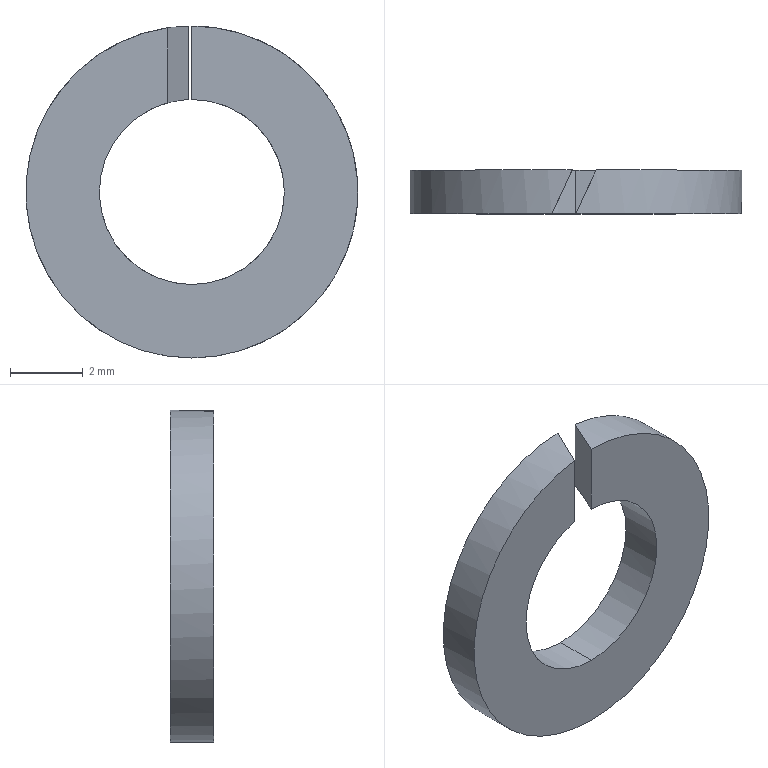Part | STEP file | M5 spring washer | 1 solid | 8 faces | box 9.15 x 1.2 x 9.15 mm | volume 52.779 mm3 | cylinder 4 | plane 4 | commonest cylinder face diameters 5.1 x2 9.15 x2
STEP:
#1=CARTESIAN_POINT('',(0.,0.,0.));
#2=DIRECTION('',(0.,0.,1.));
#3=DIRECTION('',(1.,0.,0.));
#4=AXIS2_PLACEMENT_3D('',#1,#2,#3);
#5=CARTESIAN_POINT('',(0.,0.,2.55));
#6=VERTEX_POINT('',#5);
#7=CARTESIAN_POINT('',(0.5596,1.2,2.488));
#8=VERTEX_POINT('',#7);
#9=CARTESIAN_POINT('',(0.,0.,2.55));
#10=CARTESIAN_POINT('',(0.1884,0.4041,2.55));
#11=CARTESIAN_POINT('',(0.3757,0.8057,2.529));
#12=CARTESIAN_POINT('',(0.5596,1.2,2.488));
#13=(BOUNDED_CURVE()B_SPLINE_CURVE(3,(#9,#10,#11,#12),.UNSPECIFIED.,.F.,.F.)B_SPLINE_CURVE_WITH_KNOTS((4,4),(1.571,1.792),.PIECEWISE_BEZIER_KNOTS.)CURVE()GEOMETRIC_REPRESENTATION_ITEM()RATIONAL_B_SPLINE_CURVE((1.,0.9959,0.9959,1.))REPRESENTATION_ITEM(''));
#14=CARTESIAN_POINT('',(0.,1.2,0.));
#15=DIRECTION('',(0.,-1.,0.));
#16=DIRECTION('',(0.,0.,-1.));
#17=AXIS2_PLACEMENT_3D('',#14,#15,#16);
#18=CYLINDRICAL_SURFACE('',#17,2.55);
#19=CARTESIAN_POINT('',(3.142,1.2));
#20=CARTESIAN_POINT('',(3.138,1.182));
#21=CARTESIAN_POINT('',(3.132,1.145));
#22=CARTESIAN_POINT('',(3.122,1.09));
#23=CARTESIAN_POINT('',(3.111,1.035));
#24=CARTESIAN_POINT('',(3.101,0.9803));
#25=CARTESIAN_POINT('',(3.091,0.9254));
#26=CARTESIAN_POINT('',(3.081,0.8705));
#27=CARTESIAN_POINT('',(3.071,0.8156));
#28=CARTESIAN_POINT('',(3.061,0.7607));
#29=CARTESIAN_POINT('',(3.051,0.7058));
#30=CARTESIAN_POINT('',(3.041,0.651));
#31=CARTESIAN_POINT('',(3.031,0.5963));
#32=CARTESIAN_POINT('',(3.021,0.5416));
#33=CARTESIAN_POINT('',(3.011,0.487));
#34=CARTESIAN_POINT('',(3.001,0.4325));
#35=CARTESIAN_POINT('',(2.991,0.378));
#36=CARTESIAN_POINT('',(2.981,0.3237));
#37=CARTESIAN_POINT('',(2.971,0.2694));
#38=CARTESIAN_POINT('',(2.961,0.2153));
#39=CARTESIAN_POINT('',(2.95,0.1613));
#40=CARTESIAN_POINT('',(2.94,0.1074));
#41=CARTESIAN_POINT('',(2.93,0.05359));
#42=CARTESIAN_POINT('',(2.924,0.01785));
#43=CARTESIAN_POINT('',(2.92,0.));
#44=B_SPLINE_CURVE_WITH_KNOTS('',3,(#19,#20,#21,#22,#23,#24,#25,#26,#27,#28,#29,#30,#31,#32,#33,#34,#35,#36,#37,#38,#39,#40,#41,#42,#43),.UNSPECIFIED.,.F.,.F.,(4,1,1,1,1,1,1,1,1,1,1,1,1,1,1,1,1,1,1,1,1,1,4),(1.571,1.581,1.591,1.601,1.611,1.621,1.631,1.641,1.651,1.661,1.671,1.681,1.691,1.702,1.712,1.722,1.732,1.742,1.752,1.762,1.772,1.782,1.792),.QUASI_UNIFORM_KNOTS.);
#45=(GEOMETRIC_REPRESENTATION_CONTEXT(2)PARAMETRIC_REPRESENTATION_CONTEXT()REPRESENTATION_CONTEXT('',''));
#46=DEFINITIONAL_REPRESENTATION('',(#44),#45);
#47=PCURVE('',#18,#46);
#48=CARTESIAN_POINT('',(0.,0.,4.575));
#49=DIRECTION('',(-0.9063,0.4226,0.));
#50=DIRECTION('',(-0.4226,-0.9063,0.));
#51=AXIS2_PLACEMENT_3D('',#48,#49,#50);
#52=PLANE('',#51);
#53=CARTESIAN_POINT('',(0.,-2.025));
#54=CARTESIAN_POINT('',(-0.4459,-2.025));
#55=CARTESIAN_POINT('',(-0.889,-2.046));
#56=CARTESIAN_POINT('',(-1.324,-2.087));
#57=(BOUNDED_CURVE()B_SPLINE_CURVE(3,(#53,#54,#55,#56),.UNSPECIFIED.,.F.,.F.)B_SPLINE_CURVE_WITH_KNOTS((4,4),(1.571,1.792),.PIECEWISE_BEZIER_KNOTS.)CURVE()GEOMETRIC_REPRESENTATION_ITEM()RATIONAL_B_SPLINE_CURVE((1.,0.9959,0.9959,1.))REPRESENTATION_ITEM(''));
#58=(GEOMETRIC_REPRESENTATION_CONTEXT(2)PARAMETRIC_REPRESENTATION_CONTEXT()REPRESENTATION_CONTEXT('',''));
#59=DEFINITIONAL_REPRESENTATION('',(#57),#58);
#60=PCURVE('',#52,#59);
#61=SURFACE_CURVE('',#13,(#47,#60),.PCURVE_S1.);
#62=EDGE_CURVE('',#6,#8,#61,.T.);
#63=ORIENTED_EDGE('',*,*,#62,.F.);
#64=CARTESIAN_POINT('',(0.,0.,-2.55));
#65=VERTEX_POINT('',#64);
#66=CARTESIAN_POINT('',(0.,0.,0.));
#67=DIRECTION('',(0.,1.,0.));
#68=DIRECTION('',(0.,0.,1.));
#69=AXIS2_PLACEMENT_3D('',#66,#67,#68);
#70=CIRCLE('',#69,2.55);
#71=CARTESIAN_POINT('',(3.142,1.2));
#72=DIRECTION('',(-1.,0.));
#73=VECTOR('',#72,1.);
#74=LINE('',#71,#73);
#75=(GEOMETRIC_REPRESENTATION_CONTEXT(2)PARAMETRIC_REPRESENTATION_CONTEXT()REPRESENTATION_CONTEXT('',''));
#76=DEFINITIONAL_REPRESENTATION('',(#74),#75);
#77=PCURVE('',#18,#76);
#78=CARTESIAN_POINT('',(0.,0.,0.));
#79=DIRECTION('',(0.,1.,0.));
#80=DIRECTION('',(0.,0.,1.));
#81=AXIS2_PLACEMENT_3D('',#78,#79,#80);
#82=PLANE('',#81);
#83=CARTESIAN_POINT('',(0.,0.));
#84=DIRECTION('',(1.,0.));
#85=AXIS2_PLACEMENT_2D('',#83,#84);
#86=CIRCLE('',#85,2.55);
#87=(GEOMETRIC_REPRESENTATION_CONTEXT(2)PARAMETRIC_REPRESENTATION_CONTEXT()REPRESENTATION_CONTEXT('',''));
#88=DEFINITIONAL_REPRESENTATION('',(#86),#87);
#89=PCURVE('',#82,#88);
#90=SURFACE_CURVE('',#70,(#77,#89),.PCURVE_S1.);
#91=EDGE_CURVE('',#6,#65,#90,.T.);
#92=ORIENTED_EDGE('',*,*,#91,.T.);
#93=CARTESIAN_POINT('',(0.,1.2,-2.55));
#94=VERTEX_POINT('',#93);
#95=CARTESIAN_POINT('',(0.,1.2,-2.55));
#96=DIRECTION('',(0.,-1.,0.));
#97=VECTOR('',#96,1.);
#98=LINE('',#95,#97);
#99=CARTESIAN_POINT('',(0.,0.));
#100=DIRECTION('',(0.,1.));
#101=VECTOR('',#100,1.);
#102=LINE('',#99,#101);
#103=(GEOMETRIC_REPRESENTATION_CONTEXT(2)PARAMETRIC_REPRESENTATION_CONTEXT()REPRESENTATION_CONTEXT('',''));
#104=DEFINITIONAL_REPRESENTATION('',(#102),#103);
#105=PCURVE('',#18,#104);
#106=CARTESIAN_POINT('',(0.,1.2,0.));
#107=DIRECTION('',(0.,-1.,0.));
#108=DIRECTION('',(0.,0.,-1.));
#109=AXIS2_PLACEMENT_3D('',#106,#107,#108);
#110=CYLINDRICAL_SURFACE('',#109,2.55);
#111=CARTESIAN_POINT('',(6.283,0.));
#112=DIRECTION('',(0.,1.));
#113=VECTOR('',#112,1.);
#114=LINE('',#111,#113);
#115=(GEOMETRIC_REPRESENTATION_CONTEXT(2)PARAMETRIC_REPRESENTATION_CONTEXT()REPRESENTATION_CONTEXT('',''));
#116=DEFINITIONAL_REPRESENTATION('',(#114),#115);
#117=PCURVE('',#110,#116);
#118=SURFACE_CURVE('',#98,(#105,#117),.PCURVE_S1.);
#119=EDGE_CURVE('',#94,#65,#118,.T.);
#120=ORIENTED_EDGE('',*,*,#119,.F.);
#121=CARTESIAN_POINT('',(0.,1.2,0.));
#122=DIRECTION('',(0.,1.,0.));
#123=DIRECTION('',(0.,0.,1.));
#124=AXIS2_PLACEMENT_3D('',#121,#122,#123);
#125=CIRCLE('',#124,2.55);
#126=CARTESIAN_POINT('',(3.142,0.));
#127=DIRECTION('',(-1.,0.));
#128=VECTOR('',#127,1.);
#129=LINE('',#126,#128);
#130=(GEOMETRIC_REPRESENTATION_CONTEXT(2)PARAMETRIC_REPRESENTATION_CONTEXT()REPRESENTATION_CONTEXT('',''));
#131=DEFINITIONAL_REPRESENTATION('',(#129),#130);
#132=PCURVE('',#18,#131);
#133=CARTESIAN_POINT('',(0.,1.2,0.));
#134=DIRECTION('',(0.,1.,0.));
#135=DIRECTION('',(0.,0.,1.));
#136=AXIS2_PLACEMENT_3D('',#133,#134,#135);
#137=PLANE('',#136);
#138=CARTESIAN_POINT('',(0.,0.));
#139=DIRECTION('',(1.,0.));
#140=AXIS2_PLACEMENT_2D('',#138,#139);
#141=CIRCLE('',#140,2.55);
#142=(GEOMETRIC_REPRESENTATION_CONTEXT(2)PARAMETRIC_REPRESENTATION_CONTEXT()REPRESENTATION_CONTEXT('',''));
#143=DEFINITIONAL_REPRESENTATION('',(#141),#142);
#144=PCURVE('',#137,#143);
#145=SURFACE_CURVE('',#125,(#132,#144),.PCURVE_S1.);
#146=EDGE_CURVE('',#8,#94,#145,.T.);
#147=ORIENTED_EDGE('',*,*,#146,.F.);
#148=EDGE_LOOP('',(#63,#92,#120,#147));
#149=FACE_BOUND('',#148,.F.);
#150=ADVANCED_FACE('',(#149),#18,.F.);
#151=CARTESIAN_POINT('',(0.,1.2,-4.575));
#152=VERTEX_POINT('',#151);
#153=CARTESIAN_POINT('',(-0.1025,1.2,4.574));
#154=VERTEX_POINT('',#153);
#155=CARTESIAN_POINT('',(0.,1.2,0.));
#156=DIRECTION('',(0.,1.,0.));
#157=DIRECTION('',(0.,0.,1.));
#158=AXIS2_PLACEMENT_3D('',#155,#156,#157);
#159=CIRCLE('',#158,4.575);
#160=CARTESIAN_POINT('',(0.,1.2,0.));
#161=DIRECTION('',(0.,-1.,0.));
#162=DIRECTION('',(0.,0.,-1.));
#163=AXIS2_PLACEMENT_3D('',#160,#161,#162);
#164=CYLINDRICAL_SURFACE('',#163,4.575);
#165=CARTESIAN_POINT('',(9.425,0.));
#166=DIRECTION('',(-1.,0.));
#167=VECTOR('',#166,1.);
#168=LINE('',#165,#167);
#169=(GEOMETRIC_REPRESENTATION_CONTEXT(2)PARAMETRIC_REPRESENTATION_CONTEXT()REPRESENTATION_CONTEXT('',''));
#170=DEFINITIONAL_REPRESENTATION('',(#168),#169);
#171=PCURVE('',#164,#170);
#172=CARTESIAN_POINT('',(0.,0.));
#173=DIRECTION('',(1.,0.));
#174=AXIS2_PLACEMENT_2D('',#172,#173);
#175=CIRCLE('',#174,4.575);
#176=(GEOMETRIC_REPRESENTATION_CONTEXT(2)PARAMETRIC_REPRESENTATION_CONTEXT()REPRESENTATION_CONTEXT('',''));
#177=DEFINITIONAL_REPRESENTATION('',(#175),#176);
#178=PCURVE('',#137,#177);
#179=SURFACE_CURVE('',#159,(#171,#178),.PCURVE_S1.);
#180=EDGE_CURVE('',#152,#154,#179,.T.);
#181=ORIENTED_EDGE('',*,*,#180,.F.);
#182=CARTESIAN_POINT('',(0.,0.,-4.575));
#183=VERTEX_POINT('',#182);
#184=CARTESIAN_POINT('',(0.,1.2,-4.575));
#185=DIRECTION('',(0.,-1.,0.));
#186=VECTOR('',#185,1.);
#187=LINE('',#184,#186);
#188=CARTESIAN_POINT('',(6.283,0.));
#189=DIRECTION('',(0.,1.));
#190=VECTOR('',#189,1.);
#191=LINE('',#188,#190);
#192=(GEOMETRIC_REPRESENTATION_CONTEXT(2)PARAMETRIC_REPRESENTATION_CONTEXT()REPRESENTATION_CONTEXT('',''));
#193=DEFINITIONAL_REPRESENTATION('',(#191),#192);
#194=PCURVE('',#164,#193);
#195=CARTESIAN_POINT('',(0.,1.2,0.));
#196=DIRECTION('',(0.,-1.,0.));
#197=DIRECTION('',(0.,0.,-1.));
#198=AXIS2_PLACEMENT_3D('',#195,#196,#197);
#199=CYLINDRICAL_SURFACE('',#198,4.575);
#200=CARTESIAN_POINT('',(0.,0.));
#201=DIRECTION('',(0.,1.));
#202=VECTOR('',#201,1.);
#203=LINE('',#200,#202);
#204=(GEOMETRIC_REPRESENTATION_CONTEXT(2)PARAMETRIC_REPRESENTATION_CONTEXT()REPRESENTATION_CONTEXT('',''));
#205=DEFINITIONAL_REPRESENTATION('',(#203),#204);
#206=PCURVE('',#199,#205);
#207=SURFACE_CURVE('',#187,(#194,#206),.PCURVE_S1.);
#208=EDGE_CURVE('',#152,#183,#207,.T.);
#209=ORIENTED_EDGE('',*,*,#208,.T.);
#210=CARTESIAN_POINT('',(-0.662,0.,4.527));
#211=VERTEX_POINT('',#210);
#212=CARTESIAN_POINT('',(0.,0.,0.));
#213=DIRECTION('',(0.,1.,0.));
#214=DIRECTION('',(0.,0.,1.));
#215=AXIS2_PLACEMENT_3D('',#212,#213,#214);
#216=CIRCLE('',#215,4.575);
#217=CARTESIAN_POINT('',(9.425,1.2));
#218=DIRECTION('',(-1.,0.));
#219=VECTOR('',#218,1.);
#220=LINE('',#217,#219);
#221=(GEOMETRIC_REPRESENTATION_CONTEXT(2)PARAMETRIC_REPRESENTATION_CONTEXT()REPRESENTATION_CONTEXT('',''));
#222=DEFINITIONAL_REPRESENTATION('',(#220),#221);
#223=PCURVE('',#164,#222);
#224=CARTESIAN_POINT('',(0.,0.));
#225=DIRECTION('',(1.,0.));
#226=AXIS2_PLACEMENT_2D('',#224,#225);
#227=CIRCLE('',#226,4.575);
#228=(GEOMETRIC_REPRESENTATION_CONTEXT(2)PARAMETRIC_REPRESENTATION_CONTEXT()REPRESENTATION_CONTEXT('',''));
#229=DEFINITIONAL_REPRESENTATION('',(#227),#228);
#230=PCURVE('',#82,#229);
#231=SURFACE_CURVE('',#216,(#223,#230),.PCURVE_S1.);
#232=EDGE_CURVE('',#183,#211,#231,.T.);
#233=ORIENTED_EDGE('',*,*,#232,.T.);
#234=CARTESIAN_POINT('',(-0.1025,1.2,4.574));
#235=CARTESIAN_POINT('',(-0.2898,0.7982,4.57));
#236=CARTESIAN_POINT('',(-0.4766,0.3977,4.554));
#237=CARTESIAN_POINT('',(-0.662,0.,4.527));
#238=(BOUNDED_CURVE()B_SPLINE_CURVE(3,(#234,#235,#236,#237),.UNSPECIFIED.,.F.,.F.)B_SPLINE_CURVE_WITH_KNOTS((4,4),(4.735,4.858),.PIECEWISE_BEZIER_KNOTS.)CURVE()GEOMETRIC_REPRESENTATION_ITEM()RATIONAL_B_SPLINE_CURVE((1.,0.9987,0.9987,1.))REPRESENTATION_ITEM(''));
#239=CARTESIAN_POINT('',(3.164,0.));
#240=CARTESIAN_POINT('',(3.166,0.01824));
#241=CARTESIAN_POINT('',(3.17,0.05472));
#242=CARTESIAN_POINT('',(3.175,0.1094));
#243=CARTESIAN_POINT('',(3.181,0.1642));
#244=CARTESIAN_POINT('',(3.186,0.2189));
#245=CARTESIAN_POINT('',(3.192,0.2736));
#246=CARTESIAN_POINT('',(3.197,0.3283));
#247=CARTESIAN_POINT('',(3.203,0.383));
#248=CARTESIAN_POINT('',(3.209,0.4377));
#249=CARTESIAN_POINT('',(3.214,0.4923));
#250=CARTESIAN_POINT('',(3.22,0.5469));
#251=CARTESIAN_POINT('',(3.225,0.6016));
#252=CARTESIAN_POINT('',(3.231,0.6561));
#253=CARTESIAN_POINT('',(3.237,0.7107));
#254=CARTESIAN_POINT('',(3.242,0.7652));
#255=CARTESIAN_POINT('',(3.248,0.8197));
#256=CARTESIAN_POINT('',(3.253,0.8742));
#257=CARTESIAN_POINT('',(3.259,0.9286));
#258=CARTESIAN_POINT('',(3.264,0.983));
#259=CARTESIAN_POINT('',(3.27,1.037));
#260=CARTESIAN_POINT('',(3.276,1.092));
#261=CARTESIAN_POINT('',(3.281,1.146));
#262=CARTESIAN_POINT('',(3.285,1.182));
#263=CARTESIAN_POINT('',(3.287,1.2));
#264=B_SPLINE_CURVE_WITH_KNOTS('',3,(#239,#240,#241,#242,#243,#244,#245,#246,#247,#248,#249,#250,#251,#252,#253,#254,#255,#256,#257,#258,#259,#260,#261,#262,#263),.UNSPECIFIED.,.F.,.F.,(4,1,1,1,1,1,1,1,1,1,1,1,1,1,1,1,1,1,1,1,1,1,4),(4.735,4.74,4.746,4.752,4.757,4.763,4.768,4.774,4.779,4.785,4.791,4.796,4.802,4.807,4.813,4.819,4.824,4.83,4.835,4.841,4.846,4.852,4.858),.QUASI_UNIFORM_KNOTS.);
#265=(GEOMETRIC_REPRESENTATION_CONTEXT(2)PARAMETRIC_REPRESENTATION_CONTEXT()REPRESENTATION_CONTEXT('',''));
#266=DEFINITIONAL_REPRESENTATION('',(#264),#265);
#267=PCURVE('',#164,#266);
#268=CARTESIAN_POINT('',(-0.1025,1.2,4.575));
#269=DIRECTION('',(0.9063,-0.4226,0.));
#270=DIRECTION('',(0.4226,0.9063,0.));
#271=AXIS2_PLACEMENT_3D('',#268,#269,#270);
#272=PLANE('',#271);
#273=CARTESIAN_POINT('',(0.,-0.001147));
#274=CARTESIAN_POINT('',(-0.4434,-0.005345));
#275=CARTESIAN_POINT('',(-0.8853,-0.02103));
#276=CARTESIAN_POINT('',(-1.324,-0.04815));
#277=(BOUNDED_CURVE()B_SPLINE_CURVE(3,(#273,#274,#275,#276),.UNSPECIFIED.,.F.,.F.)B_SPLINE_CURVE_WITH_KNOTS((4,4),(4.735,4.858),.PIECEWISE_BEZIER_KNOTS.)CURVE()GEOMETRIC_REPRESENTATION_ITEM()RATIONAL_B_SPLINE_CURVE((1.,0.9987,0.9987,1.))REPRESENTATION_ITEM(''));
#278=(GEOMETRIC_REPRESENTATION_CONTEXT(2)PARAMETRIC_REPRESENTATION_CONTEXT()REPRESENTATION_CONTEXT('',''));
#279=DEFINITIONAL_REPRESENTATION('',(#277),#278);
#280=PCURVE('',#272,#279);
#281=SURFACE_CURVE('',#238,(#267,#280),.PCURVE_S1.);
#282=EDGE_CURVE('',#154,#211,#281,.T.);
#283=ORIENTED_EDGE('',*,*,#282,.F.);
#284=EDGE_LOOP('',(#181,#209,#233,#283));
#285=FACE_BOUND('',#284,.T.);
#286=ADVANCED_FACE('',(#285),#164,.T.);
#287=ORIENTED_EDGE('',*,*,#146,.F.);
#288=CARTESIAN_POINT('',(0.5596,1.2,4.541));
#289=VERTEX_POINT('',#288);
#290=CARTESIAN_POINT('',(0.5596,1.2,4.575));
#291=DIRECTION('',(0.,0.,-1.));
#292=VECTOR('',#291,1.);
#293=LINE('',#290,#292);
#294=CARTESIAN_POINT('',(4.575,0.5596));
#295=DIRECTION('',(-1.,0.));
#296=VECTOR('',#295,1.);
#297=LINE('',#294,#296);
#298=(GEOMETRIC_REPRESENTATION_CONTEXT(2)PARAMETRIC_REPRESENTATION_CONTEXT()REPRESENTATION_CONTEXT('',''));
#299=DEFINITIONAL_REPRESENTATION('',(#297),#298);
#300=PCURVE('',#137,#299);
#301=CARTESIAN_POINT('',(-1.324,0.));
#302=DIRECTION('',(0.,-1.));
#303=VECTOR('',#302,1.);
#304=LINE('',#301,#303);
#305=(GEOMETRIC_REPRESENTATION_CONTEXT(2)PARAMETRIC_REPRESENTATION_CONTEXT()REPRESENTATION_CONTEXT('',''));
#306=DEFINITIONAL_REPRESENTATION('',(#304),#305);
#307=PCURVE('',#52,#306);
#308=SURFACE_CURVE('',#293,(#300,#307),.PCURVE_S1.);
#309=EDGE_CURVE('',#289,#8,#308,.T.);
#310=ORIENTED_EDGE('',*,*,#309,.F.);
#311=CARTESIAN_POINT('',(0.,1.2,0.));
#312=DIRECTION('',(0.,1.,0.));
#313=DIRECTION('',(0.,0.,1.));
#314=AXIS2_PLACEMENT_3D('',#311,#312,#313);
#315=CIRCLE('',#314,4.575);
#316=CARTESIAN_POINT('',(0.,0.));
#317=DIRECTION('',(1.,0.));
#318=AXIS2_PLACEMENT_2D('',#316,#317);
#319=CIRCLE('',#318,4.575);
#320=(GEOMETRIC_REPRESENTATION_CONTEXT(2)PARAMETRIC_REPRESENTATION_CONTEXT()REPRESENTATION_CONTEXT('',''));
#321=DEFINITIONAL_REPRESENTATION('',(#319),#320);
#322=PCURVE('',#137,#321);
#323=CARTESIAN_POINT('',(3.142,0.));
#324=DIRECTION('',(-1.,0.));
#325=VECTOR('',#324,1.);
#326=LINE('',#323,#325);
#327=(GEOMETRIC_REPRESENTATION_CONTEXT(2)PARAMETRIC_REPRESENTATION_CONTEXT()REPRESENTATION_CONTEXT('',''));
#328=DEFINITIONAL_REPRESENTATION('',(#326),#327);
#329=PCURVE('',#199,#328);
#330=SURFACE_CURVE('',#315,(#322,#329),.PCURVE_S1.);
#331=EDGE_CURVE('',#289,#152,#330,.T.);
#332=ORIENTED_EDGE('',*,*,#331,.T.);
#333=ORIENTED_EDGE('',*,*,#180,.T.);
#334=CARTESIAN_POINT('',(-0.1025,1.2,2.548));
#335=VERTEX_POINT('',#334);
#336=CARTESIAN_POINT('',(-0.1025,1.2,4.575));
#337=DIRECTION('',(0.,0.,-1.));
#338=VECTOR('',#337,1.);
#339=LINE('',#336,#338);
#340=CARTESIAN_POINT('',(4.575,-0.1025));
#341=DIRECTION('',(-1.,0.));
#342=VECTOR('',#341,1.);
#343=LINE('',#340,#342);
#344=(GEOMETRIC_REPRESENTATION_CONTEXT(2)PARAMETRIC_REPRESENTATION_CONTEXT()REPRESENTATION_CONTEXT('',''));
#345=DEFINITIONAL_REPRESENTATION('',(#343),#344);
#346=PCURVE('',#137,#345);
#347=CARTESIAN_POINT('',(0.,0.));
#348=DIRECTION('',(0.,-1.));
#349=VECTOR('',#348,1.);
#350=LINE('',#347,#349);
#351=(GEOMETRIC_REPRESENTATION_CONTEXT(2)PARAMETRIC_REPRESENTATION_CONTEXT()REPRESENTATION_CONTEXT('',''));
#352=DEFINITIONAL_REPRESENTATION('',(#350),#351);
#353=PCURVE('',#272,#352);
#354=SURFACE_CURVE('',#339,(#346,#353),.PCURVE_S1.);
#355=EDGE_CURVE('',#154,#335,#354,.T.);
#356=ORIENTED_EDGE('',*,*,#355,.T.);
#357=CARTESIAN_POINT('',(0.,1.2,0.));
#358=DIRECTION('',(0.,1.,0.));
#359=DIRECTION('',(0.,0.,1.));
#360=AXIS2_PLACEMENT_3D('',#357,#358,#359);
#361=CIRCLE('',#360,2.55);
#362=CARTESIAN_POINT('',(0.,0.));
#363=DIRECTION('',(1.,0.));
#364=AXIS2_PLACEMENT_2D('',#362,#363);
#365=CIRCLE('',#364,2.55);
#366=(GEOMETRIC_REPRESENTATION_CONTEXT(2)PARAMETRIC_REPRESENTATION_CONTEXT()REPRESENTATION_CONTEXT('',''));
#367=DEFINITIONAL_REPRESENTATION('',(#365),#366);
#368=PCURVE('',#137,#367);
#369=CARTESIAN_POINT('',(9.425,0.));
#370=DIRECTION('',(-1.,0.));
#371=VECTOR('',#370,1.);
#372=LINE('',#369,#371);
#373=(GEOMETRIC_REPRESENTATION_CONTEXT(2)PARAMETRIC_REPRESENTATION_CONTEXT()REPRESENTATION_CONTEXT('',''));
#374=DEFINITIONAL_REPRESENTATION('',(#372),#373);
#375=PCURVE('',#110,#374);
#376=SURFACE_CURVE('',#361,(#368,#375),.PCURVE_S1.);
#377=EDGE_CURVE('',#94,#335,#376,.T.);
#378=ORIENTED_EDGE('',*,*,#377,.F.);
#379=EDGE_LOOP('',(#287,#310,#332,#333,#356,#378));
#380=FACE_BOUND('',#379,.T.);
#381=ADVANCED_FACE('',(#380),#137,.T.);
#382=CARTESIAN_POINT('',(0.,0.,4.575));
#383=VERTEX_POINT('',#382);
#384=CARTESIAN_POINT('',(0.,0.,4.575));
#385=DIRECTION('',(0.,0.,-1.));
#386=VECTOR('',#385,1.);
#387=LINE('',#384,#386);
#388=CARTESIAN_POINT('',(4.575,0.));
#389=DIRECTION('',(-1.,0.));
#390=VECTOR('',#389,1.);
#391=LINE('',#388,#390);
#392=(GEOMETRIC_REPRESENTATION_CONTEXT(2)PARAMETRIC_REPRESENTATION_CONTEXT()REPRESENTATION_CONTEXT('',''));
#393=DEFINITIONAL_REPRESENTATION('',(#391),#392);
#394=PCURVE('',#82,#393);
#395=CARTESIAN_POINT('',(0.,0.));
#396=DIRECTION('',(0.,-1.));
#397=VECTOR('',#396,1.);
#398=LINE('',#395,#397);
#399=(GEOMETRIC_REPRESENTATION_CONTEXT(2)PARAMETRIC_REPRESENTATION_CONTEXT()REPRESENTATION_CONTEXT('',''));
#400=DEFINITIONAL_REPRESENTATION('',(#398),#399);
#401=PCURVE('',#52,#400);
#402=SURFACE_CURVE('',#387,(#394,#401),.PCURVE_S1.);
#403=EDGE_CURVE('',#383,#6,#402,.T.);
#404=ORIENTED_EDGE('',*,*,#403,.T.);
#405=ORIENTED_EDGE('',*,*,#91,.T.);
#406=CARTESIAN_POINT('',(-0.662,0.,2.463));
#407=VERTEX_POINT('',#406);
#408=CARTESIAN_POINT('',(0.,0.,0.));
#409=DIRECTION('',(0.,1.,0.));
#410=DIRECTION('',(0.,0.,1.));
#411=AXIS2_PLACEMENT_3D('',#408,#409,#410);
#412=CIRCLE('',#411,2.55);
#413=CARTESIAN_POINT('',(0.,0.));
#414=DIRECTION('',(1.,0.));
#415=AXIS2_PLACEMENT_2D('',#413,#414);
#416=CIRCLE('',#415,2.55);
#417=(GEOMETRIC_REPRESENTATION_CONTEXT(2)PARAMETRIC_REPRESENTATION_CONTEXT()REPRESENTATION_CONTEXT('',''));
#418=DEFINITIONAL_REPRESENTATION('',(#416),#417);
#419=PCURVE('',#82,#418);
#420=CARTESIAN_POINT('',(9.425,1.2));
#421=DIRECTION('',(-1.,0.));
#422=VECTOR('',#421,1.);
#423=LINE('',#420,#422);
#424=(GEOMETRIC_REPRESENTATION_CONTEXT(2)PARAMETRIC_REPRESENTATION_CONTEXT()REPRESENTATION_CONTEXT('',''));
#425=DEFINITIONAL_REPRESENTATION('',(#423),#424);
#426=PCURVE('',#110,#425);
#427=SURFACE_CURVE('',#412,(#419,#426),.PCURVE_S1.);
#428=EDGE_CURVE('',#65,#407,#427,.T.);
#429=ORIENTED_EDGE('',*,*,#428,.T.);
#430=CARTESIAN_POINT('',(-0.662,0.,4.575));
#431=DIRECTION('',(0.,0.,-1.));
#432=VECTOR('',#431,1.);
#433=LINE('',#430,#432);
#434=CARTESIAN_POINT('',(4.575,-0.662));
#435=DIRECTION('',(-1.,0.));
#436=VECTOR('',#435,1.);
#437=LINE('',#434,#436);
#438=(GEOMETRIC_REPRESENTATION_CONTEXT(2)PARAMETRIC_REPRESENTATION_CONTEXT()REPRESENTATION_CONTEXT('',''));
#439=DEFINITIONAL_REPRESENTATION('',(#437),#438);
#440=PCURVE('',#82,#439);
#441=CARTESIAN_POINT('',(-1.324,0.));
#442=DIRECTION('',(0.,-1.));
#443=VECTOR('',#442,1.);
#444=LINE('',#441,#443);
#445=(GEOMETRIC_REPRESENTATION_CONTEXT(2)PARAMETRIC_REPRESENTATION_CONTEXT()REPRESENTATION_CONTEXT('',''));
#446=DEFINITIONAL_REPRESENTATION('',(#444),#445);
#447=PCURVE('',#272,#446);
#448=SURFACE_CURVE('',#433,(#440,#447),.PCURVE_S1.);
#449=EDGE_CURVE('',#211,#407,#448,.T.);
#450=ORIENTED_EDGE('',*,*,#449,.F.);
#451=ORIENTED_EDGE('',*,*,#232,.F.);
#452=CARTESIAN_POINT('',(0.,0.,0.));
#453=DIRECTION('',(0.,1.,0.));
#454=DIRECTION('',(0.,0.,1.));
#455=AXIS2_PLACEMENT_3D('',#452,#453,#454);
#456=CIRCLE('',#455,4.575);
#457=CARTESIAN_POINT('',(0.,0.));
#458=DIRECTION('',(1.,0.));
#459=AXIS2_PLACEMENT_2D('',#457,#458);
#460=CIRCLE('',#459,4.575);
#461=(GEOMETRIC_REPRESENTATION_CONTEXT(2)PARAMETRIC_REPRESENTATION_CONTEXT()REPRESENTATION_CONTEXT('',''));
#462=DEFINITIONAL_REPRESENTATION('',(#460),#461);
#463=PCURVE('',#82,#462);
#464=CARTESIAN_POINT('',(3.142,1.2));
#465=DIRECTION('',(-1.,0.));
#466=VECTOR('',#465,1.);
#467=LINE('',#464,#466);
#468=(GEOMETRIC_REPRESENTATION_CONTEXT(2)PARAMETRIC_REPRESENTATION_CONTEXT()REPRESENTATION_CONTEXT('',''));
#469=DEFINITIONAL_REPRESENTATION('',(#467),#468);
#470=PCURVE('',#199,#469);
#471=SURFACE_CURVE('',#456,(#463,#470),.PCURVE_S1.);
#472=EDGE_CURVE('',#383,#183,#471,.T.);
#473=ORIENTED_EDGE('',*,*,#472,.F.);
#474=EDGE_LOOP('',(#404,#405,#429,#450,#451,#473));
#475=FACE_BOUND('',#474,.T.);
#476=ADVANCED_FACE('',(#475),#82,.F.);
#477=ORIENTED_EDGE('',*,*,#208,.F.);
#478=ORIENTED_EDGE('',*,*,#331,.F.);
#479=CARTESIAN_POINT('',(0.,0.,4.575));
#480=CARTESIAN_POINT('',(0.1871,0.4013,4.575));
#481=CARTESIAN_POINT('',(0.3739,0.8018,4.564));
#482=CARTESIAN_POINT('',(0.5596,1.2,4.541));
#483=(BOUNDED_CURVE()B_SPLINE_CURVE(3,(#479,#480,#481,#482),.UNSPECIFIED.,.F.,.F.)B_SPLINE_CURVE_WITH_KNOTS((4,4),(1.571,1.693),.PIECEWISE_BEZIER_KNOTS.)CURVE()GEOMETRIC_REPRESENTATION_ITEM()RATIONAL_B_SPLINE_CURVE((1.,0.9987,0.9987,1.))REPRESENTATION_ITEM(''));
#484=CARTESIAN_POINT('',(3.142,1.2));
#485=CARTESIAN_POINT('',(3.14,1.182));
#486=CARTESIAN_POINT('',(3.136,1.145));
#487=CARTESIAN_POINT('',(3.13,1.091));
#488=CARTESIAN_POINT('',(3.125,1.036));
#489=CARTESIAN_POINT('',(3.119,0.9814));
#490=CARTESIAN_POINT('',(3.114,0.9267));
#491=CARTESIAN_POINT('',(3.108,0.872));
#492=CARTESIAN_POINT('',(3.103,0.8174));
#493=CARTESIAN_POINT('',(3.097,0.7627));
#494=CARTESIAN_POINT('',(3.091,0.7081));
#495=CARTESIAN_POINT('',(3.086,0.6535));
#496=CARTESIAN_POINT('',(3.08,0.5989));
#497=CARTESIAN_POINT('',(3.075,0.5443));
#498=CARTESIAN_POINT('',(3.069,0.4897));
#499=CARTESIAN_POINT('',(3.064,0.4352));
#500=CARTESIAN_POINT('',(3.058,0.3807));
#501=CARTESIAN_POINT('',(3.052,0.3262));
#502=CARTESIAN_POINT('',(3.047,0.2717));
#503=CARTESIAN_POINT('',(3.041,0.2173));
#504=CARTESIAN_POINT('',(3.036,0.1629));
#505=CARTESIAN_POINT('',(3.03,0.1086));
#506=CARTESIAN_POINT('',(3.025,0.05425));
#507=CARTESIAN_POINT('',(3.021,0.01808));
#508=CARTESIAN_POINT('',(3.019,0.));
#509=B_SPLINE_CURVE_WITH_KNOTS('',3,(#484,#485,#486,#487,#488,#489,#490,#491,#492,#493,#494,#495,#496,#497,#498,#499,#500,#501,#502,#503,#504,#505,#506,#507,#508),.UNSPECIFIED.,.F.,.F.,(4,1,1,1,1,1,1,1,1,1,1,1,1,1,1,1,1,1,1,1,1,1,4),(1.571,1.576,1.582,1.588,1.593,1.599,1.604,1.61,1.615,1.621,1.627,1.632,1.638,1.643,1.649,1.654,1.66,1.666,1.671,1.677,1.682,1.688,1.693),.QUASI_UNIFORM_KNOTS.);
#510=(GEOMETRIC_REPRESENTATION_CONTEXT(2)PARAMETRIC_REPRESENTATION_CONTEXT()REPRESENTATION_CONTEXT('',''));
#511=DEFINITIONAL_REPRESENTATION('',(#509),#510);
#512=PCURVE('',#199,#511);
#513=CARTESIAN_POINT('',(0.,0.));
#514=CARTESIAN_POINT('',(-0.4427,0.));
#515=CARTESIAN_POINT('',(-0.8846,-0.01146));
#516=CARTESIAN_POINT('',(-1.324,-0.03435));
#517=(BOUNDED_CURVE()B_SPLINE_CURVE(3,(#513,#514,#515,#516),.UNSPECIFIED.,.F.,.F.)B_SPLINE_CURVE_WITH_KNOTS((4,4),(1.571,1.693),.PIECEWISE_BEZIER_KNOTS.)CURVE()GEOMETRIC_REPRESENTATION_ITEM()RATIONAL_B_SPLINE_CURVE((1.,0.9987,0.9987,1.))REPRESENTATION_ITEM(''));
#518=(GEOMETRIC_REPRESENTATION_CONTEXT(2)PARAMETRIC_REPRESENTATION_CONTEXT()REPRESENTATION_CONTEXT('',''));
#519=DEFINITIONAL_REPRESENTATION('',(#517),#518);
#520=PCURVE('',#52,#519);
#521=SURFACE_CURVE('',#483,(#512,#520),.PCURVE_S1.);
#522=EDGE_CURVE('',#383,#289,#521,.T.);
#523=ORIENTED_EDGE('',*,*,#522,.F.);
#524=ORIENTED_EDGE('',*,*,#472,.T.);
#525=EDGE_LOOP('',(#477,#478,#523,#524));
#526=FACE_BOUND('',#525,.T.);
#527=ADVANCED_FACE('',(#526),#199,.T.);
#528=ORIENTED_EDGE('',*,*,#428,.T.);
#529=CARTESIAN_POINT('',(-0.1025,1.2,2.548));
#530=CARTESIAN_POINT('',(-0.2918,0.794,2.54));
#531=CARTESIAN_POINT('',(-0.4791,0.3924,2.512));
#532=CARTESIAN_POINT('',(-0.662,0.,2.463));
#533=(BOUNDED_CURVE()B_SPLINE_CURVE(3,(#529,#530,#531,#532),.UNSPECIFIED.,.F.,.F.)B_SPLINE_CURVE_WITH_KNOTS((4,4),(4.753,4.975),.PIECEWISE_BEZIER_KNOTS.)CURVE()GEOMETRIC_REPRESENTATION_ITEM()RATIONAL_B_SPLINE_CURVE((1.,0.9959,0.9959,1.))REPRESENTATION_ITEM(''));
#534=CARTESIAN_POINT('',(3.182,0.));
#535=CARTESIAN_POINT('',(3.185,0.01838));
#536=CARTESIAN_POINT('',(3.192,0.05514));
#537=CARTESIAN_POINT('',(3.202,0.1103));
#538=CARTESIAN_POINT('',(3.212,0.1654));
#539=CARTESIAN_POINT('',(3.222,0.2205));
#540=CARTESIAN_POINT('',(3.232,0.2756));
#541=CARTESIAN_POINT('',(3.242,0.3307));
#542=CARTESIAN_POINT('',(3.253,0.3857));
#543=CARTESIAN_POINT('',(3.263,0.4406));
#544=CARTESIAN_POINT('',(3.273,0.4955));
#545=CARTESIAN_POINT('',(3.283,0.5504));
#546=CARTESIAN_POINT('',(3.293,0.6051));
#547=CARTESIAN_POINT('',(3.303,0.6598));
#548=CARTESIAN_POINT('',(3.313,0.7144));
#549=CARTESIAN_POINT('',(3.323,0.7688));
#550=CARTESIAN_POINT('',(3.333,0.8232));
#551=CARTESIAN_POINT('',(3.344,0.8775));
#552=CARTESIAN_POINT('',(3.354,0.9316));
#553=CARTESIAN_POINT('',(3.364,0.9856));
#554=CARTESIAN_POINT('',(3.374,1.039));
#555=CARTESIAN_POINT('',(3.384,1.093));
#556=CARTESIAN_POINT('',(3.394,1.147));
#557=CARTESIAN_POINT('',(3.401,1.182));
#558=CARTESIAN_POINT('',(3.404,1.2));
#559=B_SPLINE_CURVE_WITH_KNOTS('',3,(#534,#535,#536,#537,#538,#539,#540,#541,#542,#543,#544,#545,#546,#547,#548,#549,#550,#551,#552,#553,#554,#555,#556,#557,#558),.UNSPECIFIED.,.F.,.F.,(4,1,1,1,1,1,1,1,1,1,1,1,1,1,1,1,1,1,1,1,1,1,4),(4.753,4.763,4.773,4.783,4.793,4.803,4.813,4.823,4.833,4.844,4.854,4.864,4.874,4.884,4.894,4.904,4.914,4.924,4.935,4.945,4.955,4.965,4.975),.QUASI_UNIFORM_KNOTS.);
#560=(GEOMETRIC_REPRESENTATION_CONTEXT(2)PARAMETRIC_REPRESENTATION_CONTEXT()REPRESENTATION_CONTEXT('',''));
#561=DEFINITIONAL_REPRESENTATION('',(#559),#560);
#562=PCURVE('',#110,#561);
#563=CARTESIAN_POINT('',(0.,-2.027));
#564=CARTESIAN_POINT('',(-0.4479,-2.035));
#565=CARTESIAN_POINT('',(-0.8911,-2.063));
#566=CARTESIAN_POINT('',(-1.324,-2.112));
#567=(BOUNDED_CURVE()B_SPLINE_CURVE(3,(#563,#564,#565,#566),.UNSPECIFIED.,.F.,.F.)B_SPLINE_CURVE_WITH_KNOTS((4,4),(4.753,4.975),.PIECEWISE_BEZIER_KNOTS.)CURVE()GEOMETRIC_REPRESENTATION_ITEM()RATIONAL_B_SPLINE_CURVE((1.,0.9959,0.9959,1.))REPRESENTATION_ITEM(''));
#568=(GEOMETRIC_REPRESENTATION_CONTEXT(2)PARAMETRIC_REPRESENTATION_CONTEXT()REPRESENTATION_CONTEXT('',''));
#569=DEFINITIONAL_REPRESENTATION('',(#567),#568);
#570=PCURVE('',#272,#569);
#571=SURFACE_CURVE('',#533,(#562,#570),.PCURVE_S1.);
#572=EDGE_CURVE('',#335,#407,#571,.T.);
#573=ORIENTED_EDGE('',*,*,#572,.F.);
#574=ORIENTED_EDGE('',*,*,#377,.F.);
#575=ORIENTED_EDGE('',*,*,#119,.T.);
#576=EDGE_LOOP('',(#528,#573,#574,#575));
#577=FACE_BOUND('',#576,.F.);
#578=ADVANCED_FACE('',(#577),#110,.F.);
#579=ORIENTED_EDGE('',*,*,#282,.T.);
#580=ORIENTED_EDGE('',*,*,#449,.T.);
#581=ORIENTED_EDGE('',*,*,#572,.F.);
#582=ORIENTED_EDGE('',*,*,#355,.F.);
#583=EDGE_LOOP('',(#579,#580,#581,#582));
#584=FACE_BOUND('',#583,.T.);
#585=ADVANCED_FACE('',(#584),#272,.T.);
#586=ORIENTED_EDGE('',*,*,#522,.T.);
#587=ORIENTED_EDGE('',*,*,#309,.T.);
#588=ORIENTED_EDGE('',*,*,#62,.F.);
#589=ORIENTED_EDGE('',*,*,#403,.F.);
#590=EDGE_LOOP('',(#586,#587,#588,#589));
#591=FACE_BOUND('',#590,.T.);
#592=ADVANCED_FACE('',(#591),#52,.T.);
#593=CLOSED_SHELL('',(#150,#286,#381,#476,#527,#578,#585,#592));
#594=MANIFOLD_SOLID_BREP('',#593);
#595=(LENGTH_UNIT()NAMED_UNIT(*)SI_UNIT(.MILLI.,.METRE.));
#596=UNCERTAINTY_MEASURE_WITH_UNIT(LENGTH_MEASURE(0.0000001),#595,'','');
#597=(NAMED_UNIT(*)PLANE_ANGLE_UNIT()SI_UNIT($,.RADIAN.));
#598=(NAMED_UNIT(*)SI_UNIT($,.STERADIAN.)SOLID_ANGLE_UNIT());
#599=(GEOMETRIC_REPRESENTATION_CONTEXT(3)GLOBAL_UNCERTAINTY_ASSIGNED_CONTEXT((#596))GLOBAL_UNIT_ASSIGNED_CONTEXT((#595,#597,#598))REPRESENTATION_CONTEXT('',''));
#600=ADVANCED_BREP_SHAPE_REPRESENTATION('',(#4,#594),#599);